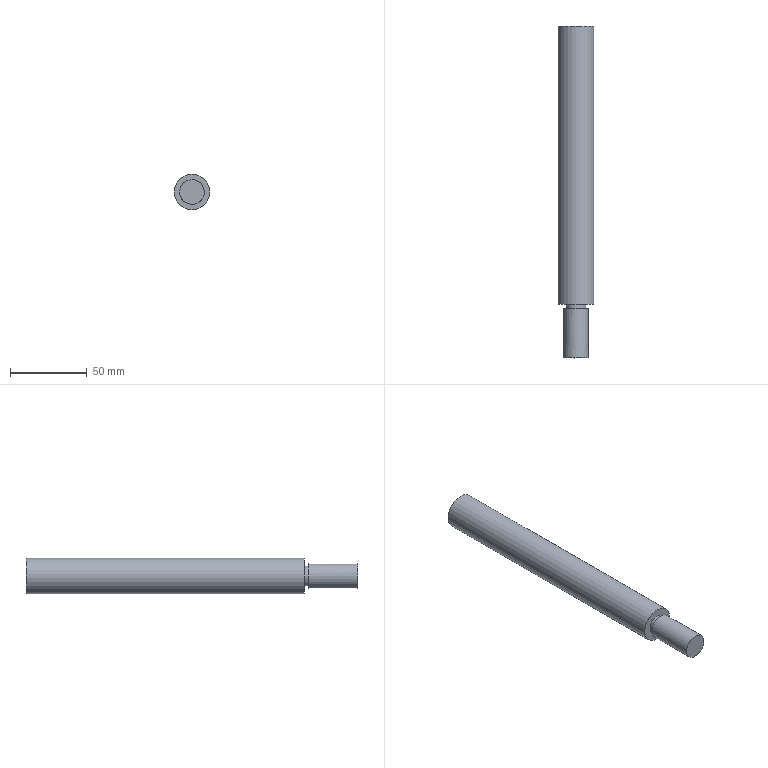Part | NX | features solid 2 | 1 solid | 9 faces | box 23 x 216 x 23 mm | volume 70854 mm3 | cylinder 4 | plane 4 | cone 1 | commonest cylinder face diameters 16 x2 13 x1 23 x1
STEP:
#1=CARTESIAN_POINT('',(-178.,812.,-370.));
#2=VERTEX_POINT('',#1);
#3=CARTESIAN_POINT('',(-170.,812.,-370.));
#4=DIRECTION('',(0.,1.,0.));
#5=DIRECTION('',(-1.,0.,0.));
#6=AXIS2_PLACEMENT_3D('',#3,#4,#5);
#7=CIRCLE('',#6,8.);
#8=EDGE_CURVE('',#2,#2,#7,.T.);
#9=ORIENTED_EDGE('',*,*,#8,.F.);
#10=EDGE_LOOP('',(#9));
#11=FACE_BOUND('',#10,.T.);
#12=CARTESIAN_POINT('',(-170.,780.,-362.));
#13=VERTEX_POINT('',#12);
#14=CARTESIAN_POINT('',(-170.,780.,-370.));
#15=DIRECTION('',(0.,1.,0.));
#16=DIRECTION('',(0.,0.,1.));
#17=AXIS2_PLACEMENT_3D('',#14,#15,#16);
#18=CIRCLE('',#17,8.);
#19=EDGE_CURVE('',#13,#13,#18,.T.);
#20=ORIENTED_EDGE('',*,*,#19,.T.);
#21=EDGE_LOOP('',(#20));
#22=FACE_BOUND('',#21,.T.);
#23=CARTESIAN_POINT('',(-170.,798.,-370.));
#24=DIRECTION('',(0.,1.,0.));
#25=DIRECTION('',(-1.,0.,0.));
#26=AXIS2_PLACEMENT_3D('',#23,#24,#25);
#27=CYLINDRICAL_SURFACE('',#26,8.);
#28=ADVANCED_FACE('',(#11,#22),#27,.T.);
#29=CARTESIAN_POINT('',(-160.34,825.,-363.76));
#30=VERTEX_POINT('',#29);
#31=CARTESIAN_POINT('',(-160.34,840.,-363.76));
#32=VERTEX_POINT('',#31);
#33=CARTESIAN_POINT('',(-160.34,967.,-363.76));
#34=DIRECTION('',(0.,-1.,0.));
#35=VECTOR('',#34,1000.);
#36=LINE('',#33,#35);
#37=EDGE_CURVE('',#30,#32,#36,.F.);
#38=ORIENTED_EDGE('',*,*,#37,.F.);
#39=ORIENTED_EDGE('',*,*,#37,.T.);
#40=EDGE_LOOP('',(#38,#39));
#41=FACE_BOUND('',#40,.T.);
#42=CARTESIAN_POINT('',(-179.66,825.,-376.24));
#43=VERTEX_POINT('',#42);
#44=CARTESIAN_POINT('',(-179.66,840.,-376.24));
#45=VERTEX_POINT('',#44);
#46=CARTESIAN_POINT('',(-179.66,967.,-376.24));
#47=DIRECTION('',(0.,-1.,0.));
#48=VECTOR('',#47,1000.);
#49=LINE('',#46,#48);
#50=EDGE_CURVE('',#43,#45,#49,.F.);
#51=ORIENTED_EDGE('',*,*,#50,.F.);
#52=ORIENTED_EDGE('',*,*,#50,.T.);
#53=EDGE_LOOP('',(#51,#52));
#54=FACE_BOUND('',#53,.T.);
#55=CARTESIAN_POINT('',(-170.,815.,-358.5));
#56=VERTEX_POINT('',#55);
#57=CARTESIAN_POINT('',(-170.,815.,-370.));
#58=DIRECTION('',(0.,1.,0.));
#59=DIRECTION('',(0.,0.,1.));
#60=AXIS2_PLACEMENT_3D('',#57,#58,#59);
#61=CIRCLE('',#60,11.5);
#62=EDGE_CURVE('',#56,#56,#61,.T.);
#63=ORIENTED_EDGE('',*,*,#62,.T.);
#64=EDGE_LOOP('',(#63));
#65=FACE_BOUND('',#64,.T.);
#66=CARTESIAN_POINT('',(-170.,996.,-358.5));
#67=VERTEX_POINT('',#66);
#68=CARTESIAN_POINT('',(-170.,996.,-370.));
#69=DIRECTION('',(0.,1.,0.));
#70=DIRECTION('',(0.,0.,1.));
#71=AXIS2_PLACEMENT_3D('',#68,#69,#70);
#72=CIRCLE('',#71,11.5);
#73=EDGE_CURVE('',#67,#67,#72,.T.);
#74=ORIENTED_EDGE('',*,*,#73,.F.);
#75=EDGE_LOOP('',(#74));
#76=FACE_BOUND('',#75,.T.);
#77=CARTESIAN_POINT('',(-160.34,825.,-376.24));
#78=VERTEX_POINT('',#77);
#79=CARTESIAN_POINT('',(-160.34,840.,-376.24));
#80=VERTEX_POINT('',#79);
#81=CARTESIAN_POINT('',(-160.34,967.,-376.24));
#82=DIRECTION('',(0.,-1.,0.));
#83=VECTOR('',#82,1000.);
#84=LINE('',#81,#83);
#85=EDGE_CURVE('',#78,#80,#84,.F.);
#86=ORIENTED_EDGE('',*,*,#85,.F.);
#87=ORIENTED_EDGE('',*,*,#85,.T.);
#88=EDGE_LOOP('',(#86,#87));
#89=FACE_BOUND('',#88,.T.);
#90=CARTESIAN_POINT('',(-179.66,825.,-363.76));
#91=VERTEX_POINT('',#90);
#92=CARTESIAN_POINT('',(-179.66,840.,-363.76));
#93=VERTEX_POINT('',#92);
#94=CARTESIAN_POINT('',(-179.66,967.,-363.76));
#95=DIRECTION('',(0.,-1.,0.));
#96=VECTOR('',#95,1000.);
#97=LINE('',#94,#96);
#98=EDGE_CURVE('',#91,#93,#97,.F.);
#99=ORIENTED_EDGE('',*,*,#98,.F.);
#100=ORIENTED_EDGE('',*,*,#98,.T.);
#101=EDGE_LOOP('',(#99,#100));
#102=FACE_BOUND('',#101,.T.);
#103=CARTESIAN_POINT('',(-170.,967.,-370.));
#104=DIRECTION('',(0.,-1.,0.));
#105=DIRECTION('',(1.,0.,0.));
#106=AXIS2_PLACEMENT_3D('',#103,#104,#105);
#107=CYLINDRICAL_SURFACE('',#106,11.5);
#108=ADVANCED_FACE('',(#41,#54,#65,#76,#89,#102),#107,.T.);
#109=CARTESIAN_POINT('',(-176.5,812.,-370.));
#110=VERTEX_POINT('',#109);
#111=CARTESIAN_POINT('',(-170.,812.,-370.));
#112=DIRECTION('',(0.,1.,0.));
#113=DIRECTION('',(-1.,0.,0.));
#114=AXIS2_PLACEMENT_3D('',#111,#112,#113);
#115=CIRCLE('',#114,6.5);
#116=EDGE_CURVE('',#110,#110,#115,.F.);
#117=ORIENTED_EDGE('',*,*,#116,.F.);
#118=EDGE_LOOP('',(#117));
#119=FACE_BOUND('',#118,.T.);
#120=CARTESIAN_POINT('',(-176.5,815.,-370.));
#121=VERTEX_POINT('',#120);
#122=CARTESIAN_POINT('',(-170.,815.,-370.));
#123=DIRECTION('',(0.,1.,0.));
#124=DIRECTION('',(-1.,0.,0.));
#125=AXIS2_PLACEMENT_3D('',#122,#123,#124);
#126=CIRCLE('',#125,6.5);
#127=EDGE_CURVE('',#121,#121,#126,.T.);
#128=ORIENTED_EDGE('',*,*,#127,.F.);
#129=EDGE_LOOP('',(#128));
#130=FACE_BOUND('',#129,.T.);
#131=CARTESIAN_POINT('',(-170.,812.,-370.));
#132=DIRECTION('',(0.,1.,0.));
#133=DIRECTION('',(-1.,0.,0.));
#134=AXIS2_PLACEMENT_3D('',#131,#132,#133);
#135=CYLINDRICAL_SURFACE('',#134,6.5);
#136=ADVANCED_FACE('',(#119,#130),#135,.T.);
#137=ORIENTED_EDGE('',*,*,#19,.F.);
#138=EDGE_LOOP('',(#137));
#139=FACE_BOUND('',#138,.T.);
#140=CARTESIAN_POINT('',(-200.,780.,-400.));
#141=DIRECTION('',(0.,1.,0.));
#142=DIRECTION('',(-1.,0.,0.));
#143=AXIS2_PLACEMENT_3D('',#140,#141,#142);
#144=PLANE('',#143);
#145=ADVANCED_FACE('',(#139),#144,.F.);
#146=ORIENTED_EDGE('',*,*,#116,.T.);
#147=EDGE_LOOP('',(#146));
#148=FACE_BOUND('',#147,.T.);
#149=ORIENTED_EDGE('',*,*,#8,.T.);
#150=EDGE_LOOP('',(#149));
#151=FACE_BOUND('',#150,.T.);
#152=CARTESIAN_POINT('',(-170.,812.,-370.));
#153=DIRECTION('',(0.,1.,0.));
#154=DIRECTION('',(-1.,0.,0.));
#155=AXIS2_PLACEMENT_3D('',#152,#153,#154);
#156=PLANE('',#155);
#157=ADVANCED_FACE('',(#148,#151),#156,.T.);
#158=ORIENTED_EDGE('',*,*,#73,.T.);
#159=EDGE_LOOP('',(#158));
#160=FACE_BOUND('',#159,.T.);
#161=CARTESIAN_POINT('',(-170.,996.,-362.));
#162=VERTEX_POINT('',#161);
#163=CARTESIAN_POINT('',(-170.,996.,-370.));
#164=DIRECTION('',(0.,1.,0.));
#165=DIRECTION('',(0.,0.,1.));
#166=AXIS2_PLACEMENT_3D('',#163,#164,#165);
#167=CIRCLE('',#166,8.);
#168=EDGE_CURVE('',#162,#162,#167,.F.);
#169=ORIENTED_EDGE('',*,*,#168,.T.);
#170=EDGE_LOOP('',(#169));
#171=FACE_BOUND('',#170,.T.);
#172=CARTESIAN_POINT('',(-170.,996.,-370.));
#173=DIRECTION('',(0.,1.,0.));
#174=DIRECTION('',(-1.,0.,0.));
#175=AXIS2_PLACEMENT_3D('',#172,#173,#174);
#176=PLANE('',#175);
#177=ADVANCED_FACE('',(#160,#171),#176,.T.);
#178=ORIENTED_EDGE('',*,*,#127,.T.);
#179=EDGE_LOOP('',(#178));
#180=FACE_BOUND('',#179,.T.);
#181=ORIENTED_EDGE('',*,*,#62,.F.);
#182=EDGE_LOOP('',(#181));
#183=FACE_BOUND('',#182,.T.);
#184=CARTESIAN_POINT('',(-170.,815.,-370.));
#185=DIRECTION('',(0.,1.,0.));
#186=DIRECTION('',(-1.,0.,0.));
#187=AXIS2_PLACEMENT_3D('',#184,#185,#186);
#188=PLANE('',#187);
#189=ADVANCED_FACE('',(#180,#183),#188,.F.);
#190=CARTESIAN_POINT('',(-162.,942.,-370.));
#191=VERTEX_POINT('',#190);
#192=CARTESIAN_POINT('',(-170.,942.,-370.));
#193=DIRECTION('',(0.,-1.,0.));
#194=DIRECTION('',(1.,0.,0.));
#195=AXIS2_PLACEMENT_3D('',#192,#193,#194);
#196=CIRCLE('',#195,8.);
#197=EDGE_CURVE('',#191,#191,#196,.T.);
#198=ORIENTED_EDGE('',*,*,#197,.F.);
#199=EDGE_LOOP('',(#198));
#200=FACE_BOUND('',#199,.T.);
#201=CARTESIAN_POINT('',(-170.,937.193,-370.));
#202=VERTEX_POINT('',#201);
#203=VERTEX_LOOP('',#202);
#204=FACE_BOUND('',#203,.T.);
#205=CARTESIAN_POINT('',(-170.,942.,-370.));
#206=DIRECTION('',(0.,1.,0.));
#207=DIRECTION('',(-1.,0.,0.));
#208=AXIS2_PLACEMENT_3D('',#205,#206,#207);
#209=CONICAL_SURFACE('',#208,8.,1.03);
#210=ADVANCED_FACE('',(#200,#204),#209,.F.);
#211=ORIENTED_EDGE('',*,*,#197,.T.);
#212=EDGE_LOOP('',(#211));
#213=FACE_BOUND('',#212,.T.);
#214=ORIENTED_EDGE('',*,*,#168,.F.);
#215=EDGE_LOOP('',(#214));
#216=FACE_BOUND('',#215,.T.);
#217=CARTESIAN_POINT('',(-170.,967.,-370.));
#218=DIRECTION('',(0.,-1.,0.));
#219=DIRECTION('',(1.,0.,0.));
#220=AXIS2_PLACEMENT_3D('',#217,#218,#219);
#221=CYLINDRICAL_SURFACE('',#220,8.);
#222=ADVANCED_FACE('',(#213,#216),#221,.F.);
#223=CLOSED_SHELL('',(#28,#108,#136,#145,#157,#177,#189,#210,#222));
#224=MANIFOLD_SOLID_BREP('',#223);
#225=(LENGTH_UNIT()NAMED_UNIT(*)SI_UNIT(.MILLI.,.METRE.));
#226=UNCERTAINTY_MEASURE_WITH_UNIT(LENGTH_MEASURE(0.00001),#225,'','');
#227=(NAMED_UNIT(*)PLANE_ANGLE_UNIT()SI_UNIT($,.RADIAN.));
#228=(NAMED_UNIT(*)SI_UNIT($,.STERADIAN.)SOLID_ANGLE_UNIT());
#229=(GEOMETRIC_REPRESENTATION_CONTEXT(3)GLOBAL_UNCERTAINTY_ASSIGNED_CONTEXT((#226))GLOBAL_UNIT_ASSIGNED_CONTEXT((#225,#227,#228))REPRESENTATION_CONTEXT('',''));
#230=ADVANCED_BREP_SHAPE_REPRESENTATION('',(#224),#229);